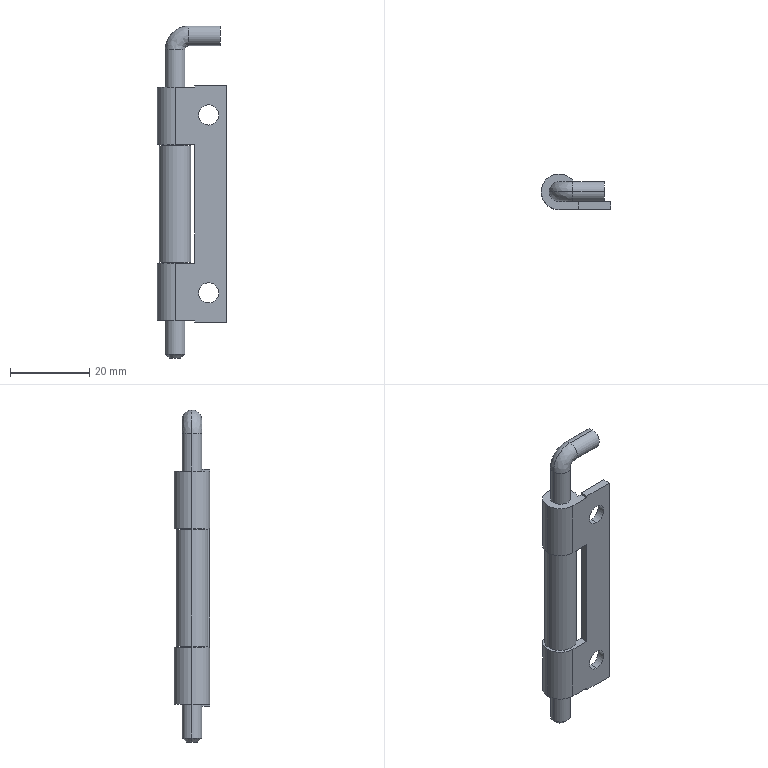Part | SolidWorks | features BaseBody 2 | 2 solids | 42 faces | box 17.6 x 9 x 84 mm | volume 4996 mm3 | cylinder 22 | plane 16 | spline 2 | cone 2 | commonest cylinder face diameters 5 x10 9 x6 5.1 x4 8 x2
STEP:
#1=CARTESIAN_POINT('',(4.5,0.,-15.));
#2=VERTEX_POINT('',#1);
#3=CARTESIAN_POINT('',(-4.5,0.,-15.));
#4=VERTEX_POINT('',#3);
#5=CARTESIAN_POINT('',(0.,0.,-15.));
#6=DIRECTION('',(0.,0.,1.));
#7=DIRECTION('',(1.,0.,0.));
#8=AXIS2_PLACEMENT_3D('',#5,#6,#7);
#9=CIRCLE('',#8,4.5);
#10=EDGE_CURVE('',#2,#4,#9,.T.);
#11=ORIENTED_EDGE('',*,*,#10,.T.);
#12=CARTESIAN_POINT('',(-4.5,0.,-0.5));
#13=VERTEX_POINT('',#12);
#14=CARTESIAN_POINT('',(-4.5,0.,0.));
#15=DIRECTION('',(0.,0.,1.));
#16=VECTOR('',#15,1000.);
#17=LINE('',#14,#16);
#18=EDGE_CURVE('',#4,#13,#17,.T.);
#19=ORIENTED_EDGE('',*,*,#18,.T.);
#20=CARTESIAN_POINT('',(4.5,0.,-0.5));
#21=VERTEX_POINT('',#20);
#22=CARTESIAN_POINT('',(0.,0.,-0.5));
#23=DIRECTION('',(0.,0.,1.));
#24=DIRECTION('',(1.,0.,0.));
#25=AXIS2_PLACEMENT_3D('',#22,#23,#24);
#26=CIRCLE('',#25,4.5);
#27=EDGE_CURVE('',#21,#13,#26,.T.);
#28=ORIENTED_EDGE('',*,*,#27,.F.);
#29=CARTESIAN_POINT('',(4.5,0.,0.));
#30=DIRECTION('',(0.,0.,1.));
#31=VECTOR('',#30,1000.);
#32=LINE('',#29,#31);
#33=EDGE_CURVE('',#2,#21,#32,.T.);
#34=ORIENTED_EDGE('',*,*,#33,.F.);
#35=EDGE_LOOP('',(#11,#19,#28,#34));
#36=FACE_OUTER_BOUND('',#35,.T.);
#37=CARTESIAN_POINT('',(0.,0.,0.));
#38=DIRECTION('',(0.,0.,1.));
#39=DIRECTION('',(1.,0.,0.));
#40=AXIS2_PLACEMENT_3D('',#37,#38,#39);
#41=CYLINDRICAL_SURFACE('',#40,4.5);
#42=ADVANCED_FACE('',(#36),#41,.T.);
#43=CARTESIAN_POINT('',(3.742,-2.5,-15.));
#44=VERTEX_POINT('',#43);
#45=CARTESIAN_POINT('',(0.,0.,-15.));
#46=DIRECTION('',(0.,0.,1.));
#47=DIRECTION('',(1.,0.,0.));
#48=AXIS2_PLACEMENT_3D('',#45,#46,#47);
#49=CIRCLE('',#48,4.5);
#50=EDGE_CURVE('',#44,#2,#49,.T.);
#51=ORIENTED_EDGE('',*,*,#50,.T.);
#52=ORIENTED_EDGE('',*,*,#33,.T.);
#53=CARTESIAN_POINT('',(3.742,-2.5,-0.5));
#54=VERTEX_POINT('',#53);
#55=CARTESIAN_POINT('',(0.,0.,-0.5));
#56=DIRECTION('',(0.,0.,1.));
#57=DIRECTION('',(1.,0.,0.));
#58=AXIS2_PLACEMENT_3D('',#55,#56,#57);
#59=CIRCLE('',#58,4.5);
#60=EDGE_CURVE('',#54,#21,#59,.T.);
#61=ORIENTED_EDGE('',*,*,#60,.F.);
#62=CARTESIAN_POINT('',(3.742,-2.5,0.));
#63=DIRECTION('',(0.,0.,-1.));
#64=VECTOR('',#63,1000.);
#65=LINE('',#62,#64);
#66=EDGE_CURVE('',#54,#44,#65,.T.);
#67=ORIENTED_EDGE('',*,*,#66,.T.);
#68=EDGE_LOOP('',(#51,#52,#61,#67));
#69=FACE_OUTER_BOUND('',#68,.T.);
#70=CARTESIAN_POINT('',(0.,0.,0.));
#71=DIRECTION('',(0.,0.,1.));
#72=DIRECTION('',(1.,0.,0.));
#73=AXIS2_PLACEMENT_3D('',#70,#71,#72);
#74=CYLINDRICAL_SURFACE('',#73,4.5);
#75=ADVANCED_FACE('',(#69),#74,.T.);
#76=CARTESIAN_POINT('',(4.5,0.,-59.5));
#77=VERTEX_POINT('',#76);
#78=CARTESIAN_POINT('',(-4.5,0.,-59.5));
#79=VERTEX_POINT('',#78);
#80=CARTESIAN_POINT('',(0.,0.,-59.5));
#81=DIRECTION('',(0.,0.,1.));
#82=DIRECTION('',(1.,0.,0.));
#83=AXIS2_PLACEMENT_3D('',#80,#81,#82);
#84=CIRCLE('',#83,4.5);
#85=EDGE_CURVE('',#77,#79,#84,.T.);
#86=ORIENTED_EDGE('',*,*,#85,.T.);
#87=CARTESIAN_POINT('',(-4.5,0.,-45.));
#88=VERTEX_POINT('',#87);
#89=CARTESIAN_POINT('',(-4.5,0.,0.));
#90=DIRECTION('',(0.,0.,1.));
#91=VECTOR('',#90,1000.);
#92=LINE('',#89,#91);
#93=EDGE_CURVE('',#79,#88,#92,.T.);
#94=ORIENTED_EDGE('',*,*,#93,.T.);
#95=CARTESIAN_POINT('',(4.5,0.,-45.));
#96=VERTEX_POINT('',#95);
#97=CARTESIAN_POINT('',(0.,0.,-45.));
#98=DIRECTION('',(0.,0.,1.));
#99=DIRECTION('',(1.,0.,0.));
#100=AXIS2_PLACEMENT_3D('',#97,#98,#99);
#101=CIRCLE('',#100,4.5);
#102=EDGE_CURVE('',#96,#88,#101,.T.);
#103=ORIENTED_EDGE('',*,*,#102,.F.);
#104=CARTESIAN_POINT('',(4.5,0.,0.));
#105=DIRECTION('',(0.,0.,1.));
#106=VECTOR('',#105,1000.);
#107=LINE('',#104,#106);
#108=EDGE_CURVE('',#77,#96,#107,.T.);
#109=ORIENTED_EDGE('',*,*,#108,.F.);
#110=EDGE_LOOP('',(#86,#94,#103,#109));
#111=FACE_OUTER_BOUND('',#110,.T.);
#112=CARTESIAN_POINT('',(0.,0.,0.));
#113=DIRECTION('',(0.,0.,1.));
#114=DIRECTION('',(1.,0.,0.));
#115=AXIS2_PLACEMENT_3D('',#112,#113,#114);
#116=CYLINDRICAL_SURFACE('',#115,4.5);
#117=ADVANCED_FACE('',(#111),#116,.T.);
#118=CARTESIAN_POINT('',(3.742,-2.5,-59.5));
#119=VERTEX_POINT('',#118);
#120=CARTESIAN_POINT('',(0.,0.,-59.5));
#121=DIRECTION('',(0.,0.,1.));
#122=DIRECTION('',(1.,0.,0.));
#123=AXIS2_PLACEMENT_3D('',#120,#121,#122);
#124=CIRCLE('',#123,4.5);
#125=EDGE_CURVE('',#119,#77,#124,.T.);
#126=ORIENTED_EDGE('',*,*,#125,.T.);
#127=ORIENTED_EDGE('',*,*,#108,.T.);
#128=CARTESIAN_POINT('',(3.742,-2.5,-45.));
#129=VERTEX_POINT('',#128);
#130=CARTESIAN_POINT('',(0.,0.,-45.));
#131=DIRECTION('',(0.,0.,1.));
#132=DIRECTION('',(1.,0.,0.));
#133=AXIS2_PLACEMENT_3D('',#130,#131,#132);
#134=CIRCLE('',#133,4.5);
#135=EDGE_CURVE('',#129,#96,#134,.T.);
#136=ORIENTED_EDGE('',*,*,#135,.F.);
#137=CARTESIAN_POINT('',(3.742,-2.5,0.));
#138=DIRECTION('',(0.,0.,-1.));
#139=VECTOR('',#138,1000.);
#140=LINE('',#137,#139);
#141=EDGE_CURVE('',#129,#119,#140,.T.);
#142=ORIENTED_EDGE('',*,*,#141,.T.);
#143=EDGE_LOOP('',(#126,#127,#136,#142));
#144=FACE_OUTER_BOUND('',#143,.T.);
#145=CARTESIAN_POINT('',(0.,0.,0.));
#146=DIRECTION('',(0.,0.,1.));
#147=DIRECTION('',(1.,0.,0.));
#148=AXIS2_PLACEMENT_3D('',#145,#146,#147);
#149=CYLINDRICAL_SURFACE('',#148,4.5);
#150=ADVANCED_FACE('',(#144),#149,.T.);
#151=CARTESIAN_POINT('',(8.5,-4.5,-4.95));
#152=VERTEX_POINT('',#151);
#153=CARTESIAN_POINT('',(8.5,-4.5,-10.05));
#154=VERTEX_POINT('',#153);
#155=CARTESIAN_POINT('',(8.5,-4.5,-7.5));
#156=DIRECTION('',(0.,-1.,0.));
#157=DIRECTION('',(0.,0.,1.));
#158=AXIS2_PLACEMENT_3D('',#155,#156,#157);
#159=CIRCLE('',#158,2.55);
#160=EDGE_CURVE('',#152,#154,#159,.T.);
#161=ORIENTED_EDGE('',*,*,#160,.T.);
#162=CARTESIAN_POINT('',(8.5,-2.5,-10.05));
#163=VERTEX_POINT('',#162);
#164=CARTESIAN_POINT('',(8.5,60.,-10.05));
#165=DIRECTION('',(0.,1.,0.));
#166=VECTOR('',#165,1000.);
#167=LINE('',#164,#166);
#168=EDGE_CURVE('',#154,#163,#167,.T.);
#169=ORIENTED_EDGE('',*,*,#168,.T.);
#170=CARTESIAN_POINT('',(8.5,-2.5,-4.95));
#171=VERTEX_POINT('',#170);
#172=CARTESIAN_POINT('',(8.5,-2.5,-7.5));
#173=DIRECTION('',(0.,-1.,0.));
#174=DIRECTION('',(0.,0.,1.));
#175=AXIS2_PLACEMENT_3D('',#172,#173,#174);
#176=CIRCLE('',#175,2.55);
#177=EDGE_CURVE('',#171,#163,#176,.T.);
#178=ORIENTED_EDGE('',*,*,#177,.F.);
#179=CARTESIAN_POINT('',(8.5,60.,-4.95));
#180=DIRECTION('',(0.,1.,0.));
#181=VECTOR('',#180,1000.);
#182=LINE('',#179,#181);
#183=EDGE_CURVE('',#152,#171,#182,.T.);
#184=ORIENTED_EDGE('',*,*,#183,.F.);
#185=EDGE_LOOP('',(#161,#169,#178,#184));
#186=FACE_OUTER_BOUND('',#185,.T.);
#187=CARTESIAN_POINT('',(8.5,60.,-7.5));
#188=DIRECTION('',(0.,1.,0.));
#189=DIRECTION('',(0.,0.,1.));
#190=AXIS2_PLACEMENT_3D('',#187,#188,#189);
#191=CYLINDRICAL_SURFACE('',#190,2.55);
#192=ADVANCED_FACE('',(#186),#191,.F.);
#193=CARTESIAN_POINT('',(8.5,-4.5,-49.95));
#194=VERTEX_POINT('',#193);
#195=CARTESIAN_POINT('',(8.5,-4.5,-55.05));
#196=VERTEX_POINT('',#195);
#197=CARTESIAN_POINT('',(8.5,-4.5,-52.5));
#198=DIRECTION('',(0.,-1.,0.));
#199=DIRECTION('',(0.,0.,1.));
#200=AXIS2_PLACEMENT_3D('',#197,#198,#199);
#201=CIRCLE('',#200,2.55);
#202=EDGE_CURVE('',#194,#196,#201,.T.);
#203=ORIENTED_EDGE('',*,*,#202,.T.);
#204=CARTESIAN_POINT('',(8.5,-2.5,-55.05));
#205=VERTEX_POINT('',#204);
#206=CARTESIAN_POINT('',(8.5,60.,-55.05));
#207=DIRECTION('',(0.,1.,0.));
#208=VECTOR('',#207,1000.);
#209=LINE('',#206,#208);
#210=EDGE_CURVE('',#196,#205,#209,.T.);
#211=ORIENTED_EDGE('',*,*,#210,.T.);
#212=CARTESIAN_POINT('',(8.5,-2.5,-49.95));
#213=VERTEX_POINT('',#212);
#214=CARTESIAN_POINT('',(8.5,-2.5,-52.5));
#215=DIRECTION('',(0.,-1.,0.));
#216=DIRECTION('',(0.,0.,1.));
#217=AXIS2_PLACEMENT_3D('',#214,#215,#216);
#218=CIRCLE('',#217,2.55);
#219=EDGE_CURVE('',#213,#205,#218,.T.);
#220=ORIENTED_EDGE('',*,*,#219,.F.);
#221=CARTESIAN_POINT('',(8.5,60.,-49.95));
#222=DIRECTION('',(0.,1.,0.));
#223=VECTOR('',#222,1000.);
#224=LINE('',#221,#223);
#225=EDGE_CURVE('',#194,#213,#224,.T.);
#226=ORIENTED_EDGE('',*,*,#225,.F.);
#227=EDGE_LOOP('',(#203,#211,#220,#226));
#228=FACE_OUTER_BOUND('',#227,.T.);
#229=CARTESIAN_POINT('',(8.5,60.,-52.5));
#230=DIRECTION('',(0.,1.,0.));
#231=DIRECTION('',(0.,0.,1.));
#232=AXIS2_PLACEMENT_3D('',#229,#230,#231);
#233=CYLINDRICAL_SURFACE('',#232,2.55);
#234=ADVANCED_FACE('',(#228),#233,.F.);
#235=CARTESIAN_POINT('',(-2.5,0.,-15.));
#236=VERTEX_POINT('',#235);
#237=CARTESIAN_POINT('',(2.5,0.,-15.));
#238=VERTEX_POINT('',#237);
#239=CARTESIAN_POINT('',(0.,0.,-15.));
#240=DIRECTION('',(0.,0.,1.));
#241=DIRECTION('',(1.,0.,0.));
#242=AXIS2_PLACEMENT_3D('',#239,#240,#241);
#243=CIRCLE('',#242,2.5);
#244=EDGE_CURVE('',#236,#238,#243,.T.);
#245=ORIENTED_EDGE('',*,*,#244,.F.);
#246=CARTESIAN_POINT('',(-2.5,0.,-0.5));
#247=VERTEX_POINT('',#246);
#248=CARTESIAN_POINT('',(-2.5,0.,0.));
#249=DIRECTION('',(0.,0.,1.));
#250=VECTOR('',#249,1000.);
#251=LINE('',#248,#250);
#252=EDGE_CURVE('',#236,#247,#251,.T.);
#253=ORIENTED_EDGE('',*,*,#252,.T.);
#254=CARTESIAN_POINT('',(2.5,0.,-0.5));
#255=VERTEX_POINT('',#254);
#256=CARTESIAN_POINT('',(0.,0.,-0.5));
#257=DIRECTION('',(0.,0.,-1.));
#258=DIRECTION('',(1.,0.,0.));
#259=AXIS2_PLACEMENT_3D('',#256,#257,#258);
#260=CIRCLE('',#259,2.5);
#261=EDGE_CURVE('',#255,#247,#260,.T.);
#262=ORIENTED_EDGE('',*,*,#261,.F.);
#263=CARTESIAN_POINT('',(2.5,0.,0.));
#264=DIRECTION('',(0.,0.,1.));
#265=VECTOR('',#264,1000.);
#266=LINE('',#263,#265);
#267=EDGE_CURVE('',#238,#255,#266,.T.);
#268=ORIENTED_EDGE('',*,*,#267,.F.);
#269=EDGE_LOOP('',(#245,#253,#262,#268));
#270=FACE_OUTER_BOUND('',#269,.T.);
#271=CARTESIAN_POINT('',(0.,0.,0.));
#272=DIRECTION('',(0.,0.,1.));
#273=DIRECTION('',(1.,0.,0.));
#274=AXIS2_PLACEMENT_3D('',#271,#272,#273);
#275=CYLINDRICAL_SURFACE('',#274,2.5);
#276=ADVANCED_FACE('',(#270),#275,.F.);
#277=CARTESIAN_POINT('',(-2.5,0.,-59.5));
#278=VERTEX_POINT('',#277);
#279=CARTESIAN_POINT('',(2.5,0.,-59.5));
#280=VERTEX_POINT('',#279);
#281=CARTESIAN_POINT('',(0.,0.,-59.5));
#282=DIRECTION('',(0.,0.,1.));
#283=DIRECTION('',(1.,0.,0.));
#284=AXIS2_PLACEMENT_3D('',#281,#282,#283);
#285=CIRCLE('',#284,2.5);
#286=EDGE_CURVE('',#278,#280,#285,.T.);
#287=ORIENTED_EDGE('',*,*,#286,.F.);
#288=CARTESIAN_POINT('',(-2.5,0.,-45.));
#289=VERTEX_POINT('',#288);
#290=CARTESIAN_POINT('',(-2.5,0.,0.));
#291=DIRECTION('',(0.,0.,1.));
#292=VECTOR('',#291,1000.);
#293=LINE('',#290,#292);
#294=EDGE_CURVE('',#278,#289,#293,.T.);
#295=ORIENTED_EDGE('',*,*,#294,.T.);
#296=CARTESIAN_POINT('',(2.5,0.,-45.));
#297=VERTEX_POINT('',#296);
#298=CARTESIAN_POINT('',(0.,0.,-45.));
#299=DIRECTION('',(0.,0.,-1.));
#300=DIRECTION('',(1.,0.,0.));
#301=AXIS2_PLACEMENT_3D('',#298,#299,#300);
#302=CIRCLE('',#301,2.5);
#303=EDGE_CURVE('',#297,#289,#302,.T.);
#304=ORIENTED_EDGE('',*,*,#303,.F.);
#305=CARTESIAN_POINT('',(2.5,0.,0.));
#306=DIRECTION('',(0.,0.,1.));
#307=VECTOR('',#306,1000.);
#308=LINE('',#305,#307);
#309=EDGE_CURVE('',#280,#297,#308,.T.);
#310=ORIENTED_EDGE('',*,*,#309,.F.);
#311=EDGE_LOOP('',(#287,#295,#304,#310));
#312=FACE_OUTER_BOUND('',#311,.T.);
#313=CARTESIAN_POINT('',(0.,0.,0.));
#314=DIRECTION('',(0.,0.,1.));
#315=DIRECTION('',(1.,0.,0.));
#316=AXIS2_PLACEMENT_3D('',#313,#314,#315);
#317=CYLINDRICAL_SURFACE('',#316,2.5);
#318=ADVANCED_FACE('',(#312),#317,.F.);
#319=CARTESIAN_POINT('',(0.,-4.5,-0.5));
#320=VERTEX_POINT('',#319);
#321=CARTESIAN_POINT('',(5.,-4.5,-0.5));
#322=VERTEX_POINT('',#321);
#323=CARTESIAN_POINT('',(0.,-4.5,-0.5));
#324=DIRECTION('',(1.,0.,0.));
#325=VECTOR('',#324,1000.);
#326=LINE('',#323,#325);
#327=EDGE_CURVE('',#320,#322,#326,.T.);
#328=ORIENTED_EDGE('',*,*,#327,.F.);
#329=CARTESIAN_POINT('',(0.,-4.5,-15.));
#330=VERTEX_POINT('',#329);
#331=CARTESIAN_POINT('',(0.,-4.5,0.));
#332=DIRECTION('',(0.,0.,1.));
#333=VECTOR('',#332,1000.);
#334=LINE('',#331,#333);
#335=EDGE_CURVE('',#330,#320,#334,.T.);
#336=ORIENTED_EDGE('',*,*,#335,.F.);
#337=CARTESIAN_POINT('',(5.,-4.5,-15.));
#338=VERTEX_POINT('',#337);
#339=CARTESIAN_POINT('',(0.,-4.5,-15.));
#340=DIRECTION('',(-1.,0.,0.));
#341=VECTOR('',#340,1000.);
#342=LINE('',#339,#341);
#343=EDGE_CURVE('',#338,#330,#342,.T.);
#344=ORIENTED_EDGE('',*,*,#343,.F.);
#345=CARTESIAN_POINT('',(5.,-4.5,-45.));
#346=VERTEX_POINT('',#345);
#347=CARTESIAN_POINT('',(5.,-4.5,0.));
#348=DIRECTION('',(0.,0.,1.));
#349=VECTOR('',#348,1000.);
#350=LINE('',#347,#349);
#351=EDGE_CURVE('',#346,#338,#350,.T.);
#352=ORIENTED_EDGE('',*,*,#351,.F.);
#353=CARTESIAN_POINT('',(0.,-4.5,-45.));
#354=VERTEX_POINT('',#353);
#355=CARTESIAN_POINT('',(0.,-4.5,-45.));
#356=DIRECTION('',(1.,0.,0.));
#357=VECTOR('',#356,1000.);
#358=LINE('',#355,#357);
#359=EDGE_CURVE('',#354,#346,#358,.T.);
#360=ORIENTED_EDGE('',*,*,#359,.F.);
#361=CARTESIAN_POINT('',(0.,-4.5,-59.5));
#362=VERTEX_POINT('',#361);
#363=CARTESIAN_POINT('',(0.,-4.5,0.));
#364=DIRECTION('',(0.,0.,1.));
#365=VECTOR('',#364,1000.);
#366=LINE('',#363,#365);
#367=EDGE_CURVE('',#362,#354,#366,.T.);
#368=ORIENTED_EDGE('',*,*,#367,.F.);
#369=CARTESIAN_POINT('',(5.,-4.5,-59.5));
#370=VERTEX_POINT('',#369);
#371=CARTESIAN_POINT('',(0.,-4.5,-59.5));
#372=DIRECTION('',(-1.,0.,0.));
#373=VECTOR('',#372,1000.);
#374=LINE('',#371,#373);
#375=EDGE_CURVE('',#370,#362,#374,.T.);
#376=ORIENTED_EDGE('',*,*,#375,.F.);
#377=CARTESIAN_POINT('',(5.,-4.5,-60.));
#378=VERTEX_POINT('',#377);
#379=CARTESIAN_POINT('',(5.,-4.5,-59.5));
#380=DIRECTION('',(0.,0.,1.));
#381=VECTOR('',#380,1000.);
#382=LINE('',#379,#381);
#383=EDGE_CURVE('',#378,#370,#382,.T.);
#384=ORIENTED_EDGE('',*,*,#383,.F.);
#385=CARTESIAN_POINT('',(13.1,-4.5,-60.));
#386=VERTEX_POINT('',#385);
#387=CARTESIAN_POINT('',(0.,-4.5,-60.));
#388=DIRECTION('',(-1.,0.,0.));
#389=VECTOR('',#388,1000.);
#390=LINE('',#387,#389);
#391=EDGE_CURVE('',#386,#378,#390,.T.);
#392=ORIENTED_EDGE('',*,*,#391,.F.);
#393=CARTESIAN_POINT('',(13.1,-4.5,0.));
#394=VERTEX_POINT('',#393);
#395=CARTESIAN_POINT('',(13.1,-4.5,0.));
#396=DIRECTION('',(0.,0.,-1.));
#397=VECTOR('',#396,1000.);
#398=LINE('',#395,#397);
#399=EDGE_CURVE('',#394,#386,#398,.T.);
#400=ORIENTED_EDGE('',*,*,#399,.F.);
#401=CARTESIAN_POINT('',(5.,-4.5,0.));
#402=VERTEX_POINT('',#401);
#403=CARTESIAN_POINT('',(0.,-4.5,0.));
#404=DIRECTION('',(1.,0.,0.));
#405=VECTOR('',#404,1000.);
#406=LINE('',#403,#405);
#407=EDGE_CURVE('',#402,#394,#406,.T.);
#408=ORIENTED_EDGE('',*,*,#407,.F.);
#409=CARTESIAN_POINT('',(5.,-4.5,0.));
#410=DIRECTION('',(0.,0.,1.));
#411=VECTOR('',#410,1000.);
#412=LINE('',#409,#411);
#413=EDGE_CURVE('',#322,#402,#412,.T.);
#414=ORIENTED_EDGE('',*,*,#413,.F.);
#415=EDGE_LOOP('',(#328,#336,#344,#352,#360,#368,#376,#384,#392,#400,#408,#414));
#416=FACE_OUTER_BOUND('',#415,.T.);
#417=ORIENTED_EDGE('',*,*,#160,.F.);
#418=CARTESIAN_POINT('',(8.5,-4.5,-7.5));
#419=DIRECTION('',(0.,-1.,0.));
#420=DIRECTION('',(0.,0.,1.));
#421=AXIS2_PLACEMENT_3D('',#418,#419,#420);
#422=CIRCLE('',#421,2.55);
#423=EDGE_CURVE('',#154,#152,#422,.T.);
#424=ORIENTED_EDGE('',*,*,#423,.F.);
#425=EDGE_LOOP('',(#417,#424));
#426=FACE_BOUND('',#425,.T.);
#427=ORIENTED_EDGE('',*,*,#202,.F.);
#428=CARTESIAN_POINT('',(8.5,-4.5,-52.5));
#429=DIRECTION('',(0.,-1.,0.));
#430=DIRECTION('',(0.,0.,1.));
#431=AXIS2_PLACEMENT_3D('',#428,#429,#430);
#432=CIRCLE('',#431,2.55);
#433=EDGE_CURVE('',#196,#194,#432,.T.);
#434=ORIENTED_EDGE('',*,*,#433,.F.);
#435=EDGE_LOOP('',(#427,#434));
#436=FACE_BOUND('',#435,.T.);
#437=CARTESIAN_POINT('',(0.,-4.5,0.));
#438=DIRECTION('',(0.,1.,0.));
#439=DIRECTION('',(0.,0.,1.));
#440=AXIS2_PLACEMENT_3D('',#437,#438,#439);
#441=PLANE('',#440);
#442=ADVANCED_FACE('',(#416,#426,#436),#441,.F.);
#443=ORIENTED_EDGE('',*,*,#327,.T.);
#444=CARTESIAN_POINT('',(5.,-2.5,-0.5));
#445=VERTEX_POINT('',#444);
#446=CARTESIAN_POINT('',(5.,60.,-0.5));
#447=DIRECTION('',(0.,1.,0.));
#448=VECTOR('',#447,1000.);
#449=LINE('',#446,#448);
#450=EDGE_CURVE('',#322,#445,#449,.T.);
#451=ORIENTED_EDGE('',*,*,#450,.T.);
#452=CARTESIAN_POINT('',(13.1,-2.5,-0.5));
#453=DIRECTION('',(-1.,0.,0.));
#454=VECTOR('',#453,1000.);
#455=LINE('',#452,#454);
#456=EDGE_CURVE('',#445,#54,#455,.T.);
#457=ORIENTED_EDGE('',*,*,#456,.T.);
#458=ORIENTED_EDGE('',*,*,#60,.T.);
#459=ORIENTED_EDGE('',*,*,#27,.T.);
#460=CARTESIAN_POINT('',(0.,0.,-0.5));
#461=DIRECTION('',(0.,0.,1.));
#462=DIRECTION('',(1.,0.,0.));
#463=AXIS2_PLACEMENT_3D('',#460,#461,#462);
#464=CIRCLE('',#463,4.5);
#465=EDGE_CURVE('',#13,#320,#464,.T.);
#466=ORIENTED_EDGE('',*,*,#465,.T.);
#467=EDGE_LOOP('',(#443,#451,#457,#458,#459,#466));
#468=FACE_OUTER_BOUND('',#467,.T.);
#469=ORIENTED_EDGE('',*,*,#261,.T.);
#470=CARTESIAN_POINT('',(0.,0.,-0.5));
#471=DIRECTION('',(0.,0.,-1.));
#472=DIRECTION('',(1.,0.,0.));
#473=AXIS2_PLACEMENT_3D('',#470,#471,#472);
#474=CIRCLE('',#473,2.5);
#475=EDGE_CURVE('',#247,#255,#474,.T.);
#476=ORIENTED_EDGE('',*,*,#475,.T.);
#477=EDGE_LOOP('',(#469,#476));
#478=FACE_BOUND('',#477,.T.);
#479=CARTESIAN_POINT('',(5.,60.,-0.5));
#480=DIRECTION('',(0.,0.,1.));
#481=DIRECTION('',(1.,0.,0.));
#482=AXIS2_PLACEMENT_3D('',#479,#480,#481);
#483=PLANE('',#482);
#484=ADVANCED_FACE('',(#468,#478),#483,.T.);
#485=ORIENTED_EDGE('',*,*,#18,.F.);
#486=CARTESIAN_POINT('',(0.,0.,-15.));
#487=DIRECTION('',(0.,0.,1.));
#488=DIRECTION('',(1.,0.,0.));
#489=AXIS2_PLACEMENT_3D('',#486,#487,#488);
#490=CIRCLE('',#489,4.5);
#491=EDGE_CURVE('',#4,#330,#490,.T.);
#492=ORIENTED_EDGE('',*,*,#491,.T.);
#493=ORIENTED_EDGE('',*,*,#335,.T.);
#494=ORIENTED_EDGE('',*,*,#465,.F.);
#495=EDGE_LOOP('',(#485,#492,#493,#494));
#496=FACE_OUTER_BOUND('',#495,.T.);
#497=CARTESIAN_POINT('',(0.,0.,0.));
#498=DIRECTION('',(0.,0.,1.));
#499=DIRECTION('',(1.,0.,0.));
#500=AXIS2_PLACEMENT_3D('',#497,#498,#499);
#501=CYLINDRICAL_SURFACE('',#500,4.5);
#502=ADVANCED_FACE('',(#496),#501,.T.);
#503=ORIENTED_EDGE('',*,*,#343,.T.);
#504=ORIENTED_EDGE('',*,*,#491,.F.);
#505=ORIENTED_EDGE('',*,*,#10,.F.);
#506=ORIENTED_EDGE('',*,*,#50,.F.);
#507=CARTESIAN_POINT('',(5.,-2.5,-15.));
#508=VERTEX_POINT('',#507);
#509=CARTESIAN_POINT('',(-15.,-2.5,-15.));
#510=DIRECTION('',(1.,0.,0.));
#511=VECTOR('',#510,1000.);
#512=LINE('',#509,#511);
#513=EDGE_CURVE('',#44,#508,#512,.T.);
#514=ORIENTED_EDGE('',*,*,#513,.T.);
#515=CARTESIAN_POINT('',(5.,60.,-15.));
#516=DIRECTION('',(0.,-1.,0.));
#517=VECTOR('',#516,1000.);
#518=LINE('',#515,#517);
#519=EDGE_CURVE('',#508,#338,#518,.T.);
#520=ORIENTED_EDGE('',*,*,#519,.T.);
#521=EDGE_LOOP('',(#503,#504,#505,#506,#514,#520));
#522=FACE_OUTER_BOUND('',#521,.T.);
#523=CARTESIAN_POINT('',(0.,0.,-15.));
#524=DIRECTION('',(0.,0.,1.));
#525=DIRECTION('',(1.,0.,0.));
#526=AXIS2_PLACEMENT_3D('',#523,#524,#525);
#527=CIRCLE('',#526,2.5);
#528=EDGE_CURVE('',#238,#236,#527,.T.);
#529=ORIENTED_EDGE('',*,*,#528,.T.);
#530=ORIENTED_EDGE('',*,*,#244,.T.);
#531=EDGE_LOOP('',(#529,#530));
#532=FACE_BOUND('',#531,.T.);
#533=CARTESIAN_POINT('',(-15.,60.,-15.));
#534=DIRECTION('',(0.,0.,-1.));
#535=DIRECTION('',(-1.,0.,0.));
#536=AXIS2_PLACEMENT_3D('',#533,#534,#535);
#537=PLANE('',#536);
#538=ADVANCED_FACE('',(#522,#532),#537,.T.);
#539=ORIENTED_EDGE('',*,*,#351,.T.);
#540=ORIENTED_EDGE('',*,*,#519,.F.);
#541=CARTESIAN_POINT('',(5.,-2.5,-45.));
#542=VERTEX_POINT('',#541);
#543=CARTESIAN_POINT('',(5.,-2.5,-15.));
#544=DIRECTION('',(0.,0.,-1.));
#545=VECTOR('',#544,1000.);
#546=LINE('',#543,#545);
#547=EDGE_CURVE('',#508,#542,#546,.T.);
#548=ORIENTED_EDGE('',*,*,#547,.T.);
#549=CARTESIAN_POINT('',(5.,60.,-45.));
#550=DIRECTION('',(0.,-1.,0.));
#551=VECTOR('',#550,1000.);
#552=LINE('',#549,#551);
#553=EDGE_CURVE('',#542,#346,#552,.T.);
#554=ORIENTED_EDGE('',*,*,#553,.T.);
#555=EDGE_LOOP('',(#539,#540,#548,#554));
#556=FACE_OUTER_BOUND('',#555,.T.);
#557=CARTESIAN_POINT('',(5.,60.,-15.));
#558=DIRECTION('',(-1.,0.,0.));
#559=DIRECTION('',(0.,0.,1.));
#560=AXIS2_PLACEMENT_3D('',#557,#558,#559);
#561=PLANE('',#560);
#562=ADVANCED_FACE('',(#556),#561,.T.);
#563=ORIENTED_EDGE('',*,*,#359,.T.);
#564=ORIENTED_EDGE('',*,*,#553,.F.);
#565=CARTESIAN_POINT('',(5.,-2.5,-45.));
#566=DIRECTION('',(-1.,0.,0.));
#567=VECTOR('',#566,1000.);
#568=LINE('',#565,#567);
#569=EDGE_CURVE('',#542,#129,#568,.T.);
#570=ORIENTED_EDGE('',*,*,#569,.T.);
#571=ORIENTED_EDGE('',*,*,#135,.T.);
#572=ORIENTED_EDGE('',*,*,#102,.T.);
#573=CARTESIAN_POINT('',(0.,0.,-45.));
#574=DIRECTION('',(0.,0.,1.));
#575=DIRECTION('',(1.,0.,0.));
#576=AXIS2_PLACEMENT_3D('',#573,#574,#575);
#577=CIRCLE('',#576,4.5);
#578=EDGE_CURVE('',#88,#354,#577,.T.);
#579=ORIENTED_EDGE('',*,*,#578,.T.);
#580=EDGE_LOOP('',(#563,#564,#570,#571,#572,#579));
#581=FACE_OUTER_BOUND('',#580,.T.);
#582=ORIENTED_EDGE('',*,*,#303,.T.);
#583=CARTESIAN_POINT('',(0.,0.,-45.));
#584=DIRECTION('',(0.,0.,-1.));
#585=DIRECTION('',(1.,0.,0.));
#586=AXIS2_PLACEMENT_3D('',#583,#584,#585);
#587=CIRCLE('',#586,2.5);
#588=EDGE_CURVE('',#289,#297,#587,.T.);
#589=ORIENTED_EDGE('',*,*,#588,.T.);
#590=EDGE_LOOP('',(#582,#589));
#591=FACE_BOUND('',#590,.T.);
#592=CARTESIAN_POINT('',(5.,60.,-45.));
#593=DIRECTION('',(0.,0.,1.));
#594=DIRECTION('',(1.,0.,0.));
#595=AXIS2_PLACEMENT_3D('',#592,#593,#594);
#596=PLANE('',#595);
#597=ADVANCED_FACE('',(#581,#591),#596,.T.);
#598=ORIENTED_EDGE('',*,*,#93,.F.);
#599=CARTESIAN_POINT('',(0.,0.,-59.5));
#600=DIRECTION('',(0.,0.,1.));
#601=DIRECTION('',(1.,0.,0.));
#602=AXIS2_PLACEMENT_3D('',#599,#600,#601);
#603=CIRCLE('',#602,4.5);
#604=EDGE_CURVE('',#79,#362,#603,.T.);
#605=ORIENTED_EDGE('',*,*,#604,.T.);
#606=ORIENTED_EDGE('',*,*,#367,.T.);
#607=ORIENTED_EDGE('',*,*,#578,.F.);
#608=EDGE_LOOP('',(#598,#605,#606,#607));
#609=FACE_OUTER_BOUND('',#608,.T.);
#610=CARTESIAN_POINT('',(0.,0.,0.));
#611=DIRECTION('',(0.,0.,1.));
#612=DIRECTION('',(1.,0.,0.));
#613=AXIS2_PLACEMENT_3D('',#610,#611,#612);
#614=CYLINDRICAL_SURFACE('',#613,4.5);
#615=ADVANCED_FACE('',(#609),#614,.T.);
#616=ORIENTED_EDGE('',*,*,#375,.T.);
#617=ORIENTED_EDGE('',*,*,#604,.F.);
#618=ORIENTED_EDGE('',*,*,#85,.F.);
#619=ORIENTED_EDGE('',*,*,#125,.F.);
#620=CARTESIAN_POINT('',(5.,-2.5,-59.5));
#621=VERTEX_POINT('',#620);
#622=CARTESIAN_POINT('',(-15.,-2.5,-59.5));
#623=DIRECTION('',(1.,0.,0.));
#624=VECTOR('',#623,1000.);
#625=LINE('',#622,#624);
#626=EDGE_CURVE('',#119,#621,#625,.T.);
#627=ORIENTED_EDGE('',*,*,#626,.T.);
#628=CARTESIAN_POINT('',(5.,60.,-59.5));
#629=DIRECTION('',(0.,-1.,0.));
#630=VECTOR('',#629,1000.);
#631=LINE('',#628,#630);
#632=EDGE_CURVE('',#621,#370,#631,.T.);
#633=ORIENTED_EDGE('',*,*,#632,.T.);
#634=EDGE_LOOP('',(#616,#617,#618,#619,#627,#633));
#635=FACE_OUTER_BOUND('',#634,.T.);
#636=CARTESIAN_POINT('',(0.,0.,-59.5));
#637=DIRECTION('',(0.,0.,1.));
#638=DIRECTION('',(1.,0.,0.));
#639=AXIS2_PLACEMENT_3D('',#636,#637,#638);
#640=CIRCLE('',#639,2.5);
#641=EDGE_CURVE('',#280,#278,#640,.T.);
#642=ORIENTED_EDGE('',*,*,#641,.T.);
#643=ORIENTED_EDGE('',*,*,#286,.T.);
#644=EDGE_LOOP('',(#642,#643));
#645=FACE_BOUND('',#644,.T.);
#646=CARTESIAN_POINT('',(-15.,60.,-59.5));
#647=DIRECTION('',(0.,0.,-1.));
#648=DIRECTION('',(-1.,0.,0.));
#649=AXIS2_PLACEMENT_3D('',#646,#647,#648);
#650=PLANE('',#649);
#651=ADVANCED_FACE('',(#635,#645),#650,.T.);
#652=CARTESIAN_POINT('',(13.1,-2.5,-60.));
#653=VERTEX_POINT('',#652);
#654=CARTESIAN_POINT('',(5.,-2.5,-60.));
#655=VERTEX_POINT('',#654);
#656=CARTESIAN_POINT('',(0.,-2.5,-60.));
#657=DIRECTION('',(-1.,0.,0.));
#658=VECTOR('',#657,1000.);
#659=LINE('',#656,#658);
#660=EDGE_CURVE('',#653,#655,#659,.T.);
#661=ORIENTED_EDGE('',*,*,#660,.F.);
#662=CARTESIAN_POINT('',(13.1,0.,-60.));
#663=DIRECTION('',(0.,1.,0.));
#664=VECTOR('',#663,1000.);
#665=LINE('',#662,#664);
#666=EDGE_CURVE('',#386,#653,#665,.T.);
#667=ORIENTED_EDGE('',*,*,#666,.F.);
#668=ORIENTED_EDGE('',*,*,#391,.T.);
#669=CARTESIAN_POINT('',(5.,0.,-60.));
#670=DIRECTION('',(0.,-1.,0.));
#671=VECTOR('',#670,1000.);
#672=LINE('',#669,#671);
#673=EDGE_CURVE('',#655,#378,#672,.T.);
#674=ORIENTED_EDGE('',*,*,#673,.F.);
#675=EDGE_LOOP('',(#661,#667,#668,#674));
#676=FACE_OUTER_BOUND('',#675,.T.);
#677=CARTESIAN_POINT('',(0.,0.,-60.));
#678=DIRECTION('',(0.,0.,1.));
#679=DIRECTION('',(1.,0.,0.));
#680=AXIS2_PLACEMENT_3D('',#677,#678,#679);
#681=PLANE('',#680);
#682=ADVANCED_FACE('',(#676),#681,.F.);
#683=CARTESIAN_POINT('',(13.1,-2.5,0.));
#684=VERTEX_POINT('',#683);
#685=CARTESIAN_POINT('',(13.1,-2.5,0.));
#686=DIRECTION('',(0.,0.,-1.));
#687=VECTOR('',#686,1000.);
#688=LINE('',#685,#687);
#689=EDGE_CURVE('',#684,#653,#688,.T.);
#690=ORIENTED_EDGE('',*,*,#689,.F.);
#691=CARTESIAN_POINT('',(13.1,-4.5,0.));
#692=DIRECTION('',(0.,1.,0.));
#693=VECTOR('',#692,1000.);
#694=LINE('',#691,#693);
#695=EDGE_CURVE('',#394,#684,#694,.T.);
#696=ORIENTED_EDGE('',*,*,#695,.F.);
#697=ORIENTED_EDGE('',*,*,#399,.T.);
#698=ORIENTED_EDGE('',*,*,#666,.T.);
#699=EDGE_LOOP('',(#690,#696,#697,#698));
#700=FACE_OUTER_BOUND('',#699,.T.);
#701=CARTESIAN_POINT('',(13.1,-4.5,0.));
#702=DIRECTION('',(-1.,0.,0.));
#703=DIRECTION('',(0.,0.,1.));
#704=AXIS2_PLACEMENT_3D('',#701,#702,#703);
#705=PLANE('',#704);
#706=ADVANCED_FACE('',(#700),#705,.F.);
#707=ORIENTED_EDGE('',*,*,#407,.T.);
#708=ORIENTED_EDGE('',*,*,#695,.T.);
#709=CARTESIAN_POINT('',(5.,-2.5,0.));
#710=VERTEX_POINT('',#709);
#711=CARTESIAN_POINT('',(0.,-2.5,0.));
#712=DIRECTION('',(-1.,0.,0.));
#713=VECTOR('',#712,1000.);
#714=LINE('',#711,#713);
#715=EDGE_CURVE('',#684,#710,#714,.T.);
#716=ORIENTED_EDGE('',*,*,#715,.T.);
#717=CARTESIAN_POINT('',(5.,0.,0.));
#718=DIRECTION('',(0.,-1.,0.));
#719=VECTOR('',#718,1000.);
#720=LINE('',#717,#719);
#721=EDGE_CURVE('',#710,#402,#720,.T.);
#722=ORIENTED_EDGE('',*,*,#721,.T.);
#723=EDGE_LOOP('',(#707,#708,#716,#722));
#724=FACE_OUTER_BOUND('',#723,.T.);
#725=CARTESIAN_POINT('',(0.,0.,0.));
#726=DIRECTION('',(0.,0.,1.));
#727=DIRECTION('',(1.,0.,0.));
#728=AXIS2_PLACEMENT_3D('',#725,#726,#727);
#729=PLANE('',#728);
#730=ADVANCED_FACE('',(#724),#729,.T.);
#731=ORIENTED_EDGE('',*,*,#168,.F.);
#732=ORIENTED_EDGE('',*,*,#423,.T.);
#733=ORIENTED_EDGE('',*,*,#183,.T.);
#734=CARTESIAN_POINT('',(8.5,-2.5,-7.5));
#735=DIRECTION('',(0.,-1.,0.));
#736=DIRECTION('',(0.,0.,1.));
#737=AXIS2_PLACEMENT_3D('',#734,#735,#736);
#738=CIRCLE('',#737,2.55);
#739=EDGE_CURVE('',#163,#171,#738,.T.);
#740=ORIENTED_EDGE('',*,*,#739,.F.);
#741=EDGE_LOOP('',(#731,#732,#733,#740));
#742=FACE_OUTER_BOUND('',#741,.T.);
#743=CARTESIAN_POINT('',(8.5,60.,-7.5));
#744=DIRECTION('',(0.,1.,0.));
#745=DIRECTION('',(0.,0.,1.));
#746=AXIS2_PLACEMENT_3D('',#743,#744,#745);
#747=CYLINDRICAL_SURFACE('',#746,2.55);
#748=ADVANCED_FACE('',(#742),#747,.F.);
#749=ORIENTED_EDGE('',*,*,#210,.F.);
#750=ORIENTED_EDGE('',*,*,#433,.T.);
#751=ORIENTED_EDGE('',*,*,#225,.T.);
#752=CARTESIAN_POINT('',(8.5,-2.5,-52.5));
#753=DIRECTION('',(0.,-1.,0.));
#754=DIRECTION('',(0.,0.,1.));
#755=AXIS2_PLACEMENT_3D('',#752,#753,#754);
#756=CIRCLE('',#755,2.55);
#757=EDGE_CURVE('',#205,#213,#756,.T.);
#758=ORIENTED_EDGE('',*,*,#757,.F.);
#759=EDGE_LOOP('',(#749,#750,#751,#758));
#760=FACE_OUTER_BOUND('',#759,.T.);
#761=CARTESIAN_POINT('',(8.5,60.,-52.5));
#762=DIRECTION('',(0.,1.,0.));
#763=DIRECTION('',(0.,0.,1.));
#764=AXIS2_PLACEMENT_3D('',#761,#762,#763);
#765=CYLINDRICAL_SURFACE('',#764,2.55);
#766=ADVANCED_FACE('',(#760),#765,.F.);
#767=ORIENTED_EDGE('',*,*,#413,.T.);
#768=ORIENTED_EDGE('',*,*,#721,.F.);
#769=CARTESIAN_POINT('',(5.,-2.5,0.));
#770=DIRECTION('',(0.,0.,-1.));
#771=VECTOR('',#770,1000.);
#772=LINE('',#769,#771);
#773=EDGE_CURVE('',#710,#445,#772,.T.);
#774=ORIENTED_EDGE('',*,*,#773,.T.);
#775=ORIENTED_EDGE('',*,*,#450,.F.);
#776=EDGE_LOOP('',(#767,#768,#774,#775));
#777=FACE_OUTER_BOUND('',#776,.T.);
#778=CARTESIAN_POINT('',(5.,60.,0.));
#779=DIRECTION('',(-1.,0.,0.));
#780=DIRECTION('',(0.,0.,1.));
#781=AXIS2_PLACEMENT_3D('',#778,#779,#780);
#782=PLANE('',#781);
#783=ADVANCED_FACE('',(#777),#782,.T.);
#784=ORIENTED_EDGE('',*,*,#252,.F.);
#785=ORIENTED_EDGE('',*,*,#528,.F.);
#786=ORIENTED_EDGE('',*,*,#267,.T.);
#787=ORIENTED_EDGE('',*,*,#475,.F.);
#788=EDGE_LOOP('',(#784,#785,#786,#787));
#789=FACE_OUTER_BOUND('',#788,.T.);
#790=CARTESIAN_POINT('',(0.,0.,0.));
#791=DIRECTION('',(0.,0.,1.));
#792=DIRECTION('',(1.,0.,0.));
#793=AXIS2_PLACEMENT_3D('',#790,#791,#792);
#794=CYLINDRICAL_SURFACE('',#793,2.5);
#795=ADVANCED_FACE('',(#789),#794,.F.);
#796=ORIENTED_EDGE('',*,*,#715,.F.);
#797=ORIENTED_EDGE('',*,*,#689,.T.);
#798=ORIENTED_EDGE('',*,*,#660,.T.);
#799=CARTESIAN_POINT('',(5.,-2.5,0.));
#800=DIRECTION('',(0.,0.,-1.));
#801=VECTOR('',#800,1000.);
#802=LINE('',#799,#801);
#803=EDGE_CURVE('',#621,#655,#802,.T.);
#804=ORIENTED_EDGE('',*,*,#803,.F.);
#805=ORIENTED_EDGE('',*,*,#626,.F.);
#806=ORIENTED_EDGE('',*,*,#141,.F.);
#807=ORIENTED_EDGE('',*,*,#569,.F.);
#808=ORIENTED_EDGE('',*,*,#547,.F.);
#809=ORIENTED_EDGE('',*,*,#513,.F.);
#810=ORIENTED_EDGE('',*,*,#66,.F.);
#811=ORIENTED_EDGE('',*,*,#456,.F.);
#812=ORIENTED_EDGE('',*,*,#773,.F.);
#813=EDGE_LOOP('',(#796,#797,#798,#804,#805,#806,#807,#808,#809,#810,#811,#812));
#814=FACE_OUTER_BOUND('',#813,.T.);
#815=ORIENTED_EDGE('',*,*,#177,.T.);
#816=ORIENTED_EDGE('',*,*,#739,.T.);
#817=EDGE_LOOP('',(#815,#816));
#818=FACE_BOUND('',#817,.T.);
#819=ORIENTED_EDGE('',*,*,#219,.T.);
#820=ORIENTED_EDGE('',*,*,#757,.T.);
#821=EDGE_LOOP('',(#819,#820));
#822=FACE_BOUND('',#821,.T.);
#823=CARTESIAN_POINT('',(13.1,-2.5,0.));
#824=DIRECTION('',(0.,-1.,0.));
#825=DIRECTION('',(0.,0.,-1.));
#826=AXIS2_PLACEMENT_3D('',#823,#824,#825);
#827=PLANE('',#826);
#828=ADVANCED_FACE('',(#814,#818,#822),#827,.F.);
#829=ORIENTED_EDGE('',*,*,#294,.F.);
#830=ORIENTED_EDGE('',*,*,#641,.F.);
#831=ORIENTED_EDGE('',*,*,#309,.T.);
#832=ORIENTED_EDGE('',*,*,#588,.F.);
#833=EDGE_LOOP('',(#829,#830,#831,#832));
#834=FACE_OUTER_BOUND('',#833,.T.);
#835=CARTESIAN_POINT('',(0.,0.,0.));
#836=DIRECTION('',(0.,0.,1.));
#837=DIRECTION('',(1.,0.,0.));
#838=AXIS2_PLACEMENT_3D('',#835,#836,#837);
#839=CYLINDRICAL_SURFACE('',#838,2.5);
#840=ADVANCED_FACE('',(#834),#839,.F.);
#841=ORIENTED_EDGE('',*,*,#383,.T.);
#842=ORIENTED_EDGE('',*,*,#632,.F.);
#843=ORIENTED_EDGE('',*,*,#803,.T.);
#844=ORIENTED_EDGE('',*,*,#673,.T.);
#845=EDGE_LOOP('',(#841,#842,#843,#844));
#846=FACE_OUTER_BOUND('',#845,.T.);
#847=CARTESIAN_POINT('',(5.,60.,-59.5));
#848=DIRECTION('',(-1.,0.,0.));
#849=DIRECTION('',(0.,0.,1.));
#850=AXIS2_PLACEMENT_3D('',#847,#848,#849);
#851=PLANE('',#850);
#852=ADVANCED_FACE('',(#846),#851,.T.);
#853=CLOSED_SHELL('',(#42,#75,#117,#150,#192,#234,#276,#318,#442,#484,#502,#538,#562,#597,#615,#651,#682,#706,#730,#748,#766,#783,#795,#828,#840,#852));
#854=MANIFOLD_SOLID_BREP('',#853);
#855=CARTESIAN_POINT('',(4.,0.,-15.25));
#856=VERTEX_POINT('',#855);
#857=CARTESIAN_POINT('',(-4.,0.,-15.25));
#858=VERTEX_POINT('',#857);
#859=CARTESIAN_POINT('',(0.,0.,-15.25));
#860=DIRECTION('',(0.,0.,-1.));
#861=DIRECTION('',(1.,0.,0.));
#862=AXIS2_PLACEMENT_3D('',#859,#860,#861);
#863=CIRCLE('',#862,4.);
#864=EDGE_CURVE('',#856,#858,#863,.T.);
#865=ORIENTED_EDGE('',*,*,#864,.T.);
#866=CARTESIAN_POINT('',(-4.,0.,-44.75));
#867=VERTEX_POINT('',#866);
#868=CARTESIAN_POINT('',(-4.,0.,-44.75));
#869=DIRECTION('',(0.,0.,-1.));
#870=VECTOR('',#869,1000.);
#871=LINE('',#868,#870);
#872=EDGE_CURVE('',#858,#867,#871,.T.);
#873=ORIENTED_EDGE('',*,*,#872,.T.);
#874=CARTESIAN_POINT('',(4.,0.,-44.75));
#875=VERTEX_POINT('',#874);
#876=CARTESIAN_POINT('',(0.,0.,-44.75));
#877=DIRECTION('',(0.,0.,1.));
#878=DIRECTION('',(1.,0.,0.));
#879=AXIS2_PLACEMENT_3D('',#876,#877,#878);
#880=CIRCLE('',#879,4.);
#881=EDGE_CURVE('',#867,#875,#880,.T.);
#882=ORIENTED_EDGE('',*,*,#881,.T.);
#883=CARTESIAN_POINT('',(4.,0.,-44.75));
#884=DIRECTION('',(0.,0.,-1.));
#885=VECTOR('',#884,1000.);
#886=LINE('',#883,#885);
#887=EDGE_CURVE('',#856,#875,#886,.T.);
#888=ORIENTED_EDGE('',*,*,#887,.F.);
#889=EDGE_LOOP('',(#865,#873,#882,#888));
#890=FACE_OUTER_BOUND('',#889,.T.);
#891=CARTESIAN_POINT('',(0.,0.,-44.75));
#892=DIRECTION('',(0.,0.,-1.));
#893=DIRECTION('',(1.,0.,0.));
#894=AXIS2_PLACEMENT_3D('',#891,#892,#893);
#895=CYLINDRICAL_SURFACE('',#894,4.);
#896=ADVANCED_FACE('',(#890),#895,.T.);
#897=CARTESIAN_POINT('',(2.5,0.,9.));
#898=VERTEX_POINT('',#897);
#899=CARTESIAN_POINT('',(-2.5,0.,9.));
#900=VERTEX_POINT('',#899);
#901=CARTESIAN_POINT('',(0.,0.,9.));
#902=DIRECTION('',(0.,0.,-1.));
#903=DIRECTION('',(1.,0.,0.));
#904=AXIS2_PLACEMENT_3D('',#901,#902,#903);
#905=CIRCLE('',#904,2.5);
#906=EDGE_CURVE('',#898,#900,#905,.T.);
#907=ORIENTED_EDGE('',*,*,#906,.T.);
#908=CARTESIAN_POINT('',(-2.5,0.,-15.25));
#909=VERTEX_POINT('',#908);
#910=CARTESIAN_POINT('',(-2.5,0.,-69.));
#911=DIRECTION('',(0.,0.,-1.));
#912=VECTOR('',#911,1000.);
#913=LINE('',#910,#912);
#914=EDGE_CURVE('',#900,#909,#913,.T.);
#915=ORIENTED_EDGE('',*,*,#914,.T.);
#916=CARTESIAN_POINT('',(2.5,0.,-15.25));
#917=VERTEX_POINT('',#916);
#918=CARTESIAN_POINT('',(0.,0.,-15.25));
#919=DIRECTION('',(0.,0.,1.));
#920=DIRECTION('',(1.,0.,0.));
#921=AXIS2_PLACEMENT_3D('',#918,#919,#920);
#922=CIRCLE('',#921,2.5);
#923=EDGE_CURVE('',#909,#917,#922,.T.);
#924=ORIENTED_EDGE('',*,*,#923,.T.);
#925=CARTESIAN_POINT('',(2.5,0.,-69.));
#926=DIRECTION('',(0.,0.,-1.));
#927=VECTOR('',#926,1000.);
#928=LINE('',#925,#927);
#929=EDGE_CURVE('',#898,#917,#928,.T.);
#930=ORIENTED_EDGE('',*,*,#929,.F.);
#931=EDGE_LOOP('',(#907,#915,#924,#930));
#932=FACE_OUTER_BOUND('',#931,.T.);
#933=CARTESIAN_POINT('',(0.,0.,-69.));
#934=DIRECTION('',(0.,0.,-1.));
#935=DIRECTION('',(1.,0.,0.));
#936=AXIS2_PLACEMENT_3D('',#933,#934,#935);
#937=CYLINDRICAL_SURFACE('',#936,2.5);
#938=ADVANCED_FACE('',(#932),#937,.T.);
#939=CARTESIAN_POINT('',(-2.5,0.,-44.75));
#940=VERTEX_POINT('',#939);
#941=CARTESIAN_POINT('',(2.5,0.,-44.75));
#942=VERTEX_POINT('',#941);
#943=CARTESIAN_POINT('',(0.,0.,-44.75));
#944=DIRECTION('',(0.,0.,1.));
#945=DIRECTION('',(1.,0.,0.));
#946=AXIS2_PLACEMENT_3D('',#943,#944,#945);
#947=CIRCLE('',#946,2.5);
#948=EDGE_CURVE('',#940,#942,#947,.T.);
#949=ORIENTED_EDGE('',*,*,#948,.F.);
#950=CARTESIAN_POINT('',(-2.5,0.,-68.));
#951=VERTEX_POINT('',#950);
#952=CARTESIAN_POINT('',(-2.5,0.,-69.));
#953=DIRECTION('',(0.,0.,-1.));
#954=VECTOR('',#953,1000.);
#955=LINE('',#952,#954);
#956=EDGE_CURVE('',#940,#951,#955,.T.);
#957=ORIENTED_EDGE('',*,*,#956,.T.);
#958=CARTESIAN_POINT('',(2.5,0.,-68.));
#959=VERTEX_POINT('',#958);
#960=CARTESIAN_POINT('',(0.,0.,-68.));
#961=DIRECTION('',(0.,0.,1.));
#962=DIRECTION('',(1.,0.,0.));
#963=AXIS2_PLACEMENT_3D('',#960,#961,#962);
#964=CIRCLE('',#963,2.5);
#965=EDGE_CURVE('',#951,#959,#964,.T.);
#966=ORIENTED_EDGE('',*,*,#965,.T.);
#967=CARTESIAN_POINT('',(2.5,0.,-69.));
#968=DIRECTION('',(0.,0.,-1.));
#969=VECTOR('',#968,1000.);
#970=LINE('',#967,#969);
#971=EDGE_CURVE('',#942,#959,#970,.T.);
#972=ORIENTED_EDGE('',*,*,#971,.F.);
#973=EDGE_LOOP('',(#949,#957,#966,#972));
#974=FACE_OUTER_BOUND('',#973,.T.);
#975=CARTESIAN_POINT('',(0.,0.,-69.));
#976=DIRECTION('',(0.,0.,-1.));
#977=DIRECTION('',(1.,0.,0.));
#978=AXIS2_PLACEMENT_3D('',#975,#976,#977);
#979=CYLINDRICAL_SURFACE('',#978,2.5);
#980=ADVANCED_FACE('',(#974),#979,.T.);
#981=ORIENTED_EDGE('',*,*,#906,.F.);
#982=CARTESIAN_POINT('',(3.5,0.,10.));
#983=VERTEX_POINT('',#982);
#984=CARTESIAN_POINT('',(3.5,0.,9.));
#985=DIRECTION('',(0.,1.,0.));
#986=DIRECTION('',(0.,0.,1.));
#987=AXIS2_PLACEMENT_3D('',#984,#985,#986);
#988=CIRCLE('',#987,1.);
#989=EDGE_CURVE('',#898,#983,#988,.T.);
#990=ORIENTED_EDGE('',*,*,#989,.T.);
#991=CARTESIAN_POINT('',(3.5,0.,15.));
#992=VERTEX_POINT('',#991);
#993=CARTESIAN_POINT('',(3.5,0.,12.5));
#994=DIRECTION('',(-1.,0.,0.));
#995=DIRECTION('',(0.,0.,1.));
#996=AXIS2_PLACEMENT_3D('',#993,#994,#995);
#997=CIRCLE('',#996,2.5);
#998=EDGE_CURVE('',#983,#992,#997,.T.);
#999=ORIENTED_EDGE('',*,*,#998,.T.);
#1000=CARTESIAN_POINT('',(3.5,0.,9.));
#1001=DIRECTION('',(0.,1.,0.));
#1002=DIRECTION('',(0.,0.,1.));
#1003=AXIS2_PLACEMENT_3D('',#1000,#1001,#1002);
#1004=CIRCLE('',#1003,6.);
#1005=EDGE_CURVE('',#900,#992,#1004,.T.);
#1006=ORIENTED_EDGE('',*,*,#1005,.F.);
#1007=EDGE_LOOP('',(#981,#990,#999,#1006));
#1008=FACE_OUTER_BOUND('',#1007,.T.);
#1009=CARTESIAN_POINT('',(-2.5,0.,9.));
#1010=CARTESIAN_POINT('',(-2.5,0.,12.515));
#1011=CARTESIAN_POINT('',(-0.01472,0.,15.));
#1012=CARTESIAN_POINT('',(3.5,0.,15.));
#1013=CARTESIAN_POINT('',(-2.5,-5.,9.));
#1014=CARTESIAN_POINT('',(-2.5,-5.,12.515));
#1015=CARTESIAN_POINT('',(-0.01472,-5.,15.));
#1016=CARTESIAN_POINT('',(3.5,-5.,15.));
#1017=CARTESIAN_POINT('',(2.5,-5.,9.));
#1018=CARTESIAN_POINT('',(2.5,-5.,9.586));
#1019=CARTESIAN_POINT('',(2.914,-5.,10.));
#1020=CARTESIAN_POINT('',(3.5,-5.,10.));
#1021=CARTESIAN_POINT('',(2.5,0.,9.));
#1022=CARTESIAN_POINT('',(2.5,0.,9.586));
#1023=CARTESIAN_POINT('',(2.914,0.,10.));
#1024=CARTESIAN_POINT('',(3.5,0.,10.));
#1025=(BOUNDED_SURFACE()B_SPLINE_SURFACE(3,3,((#1009,#1010,#1011,#1012),(#1013,#1014,#1015,#1016),(#1017,#1018,#1019,#1020),(#1021,#1022,#1023,#1024)),.UNSPECIFIED.,.F.,.F.,.F.)B_SPLINE_SURFACE_WITH_KNOTS((4,4),(4,4),(0.,1.),(0.,1.),.UNSPECIFIED.)GEOMETRIC_REPRESENTATION_ITEM()RATIONAL_B_SPLINE_SURFACE(((1.,0.8047,0.8047,1.),(0.3333,0.2682,0.2682,0.3333),(0.3333,0.2682,0.2682,0.3333),(1.,0.8047,0.8047,1.)))REPRESENTATION_ITEM('')SURFACE());
#1026=ADVANCED_FACE('',(#1008),#1025,.T.);
#1027=CARTESIAN_POINT('',(-1.5,0.,-69.));
#1028=VERTEX_POINT('',#1027);
#1029=CARTESIAN_POINT('',(1.5,0.,-69.));
#1030=VERTEX_POINT('',#1029);
#1031=CARTESIAN_POINT('',(0.,0.,-69.));
#1032=DIRECTION('',(0.,0.,1.));
#1033=DIRECTION('',(-1.,0.,0.));
#1034=AXIS2_PLACEMENT_3D('',#1031,#1032,#1033);
#1035=CIRCLE('',#1034,1.5);
#1036=EDGE_CURVE('',#1028,#1030,#1035,.T.);
#1037=ORIENTED_EDGE('',*,*,#1036,.T.);
#1038=CARTESIAN_POINT('',(2.5,0.,-68.));
#1039=DIRECTION('',(0.7071,0.,0.7071));
#1040=VECTOR('',#1039,1000.);
#1041=LINE('',#1038,#1040);
#1042=EDGE_CURVE('',#1030,#959,#1041,.T.);
#1043=ORIENTED_EDGE('',*,*,#1042,.T.);
#1044=ORIENTED_EDGE('',*,*,#965,.F.);
#1045=CARTESIAN_POINT('',(-2.5,0.,-68.));
#1046=DIRECTION('',(-0.7071,0.,0.7071));
#1047=VECTOR('',#1046,1000.);
#1048=LINE('',#1045,#1047);
#1049=EDGE_CURVE('',#1028,#951,#1048,.T.);
#1050=ORIENTED_EDGE('',*,*,#1049,.F.);
#1051=EDGE_LOOP('',(#1037,#1043,#1044,#1050));
#1052=FACE_OUTER_BOUND('',#1051,.T.);
#1053=CARTESIAN_POINT('',(0.,0.,-68.));
#1054=DIRECTION('',(0.,0.,1.));
#1055=DIRECTION('',(-1.,0.,0.));
#1056=AXIS2_PLACEMENT_3D('',#1053,#1054,#1055);
#1057=CONICAL_SURFACE('',#1056,2.5,0.7854);
#1058=ADVANCED_FACE('',(#1052),#1057,.T.);
#1059=ORIENTED_EDGE('',*,*,#998,.F.);
#1060=CARTESIAN_POINT('',(11.5,0.,10.));
#1061=VERTEX_POINT('',#1060);
#1062=CARTESIAN_POINT('',(11.5,0.,10.));
#1063=DIRECTION('',(1.,0.,0.));
#1064=VECTOR('',#1063,1000.);
#1065=LINE('',#1062,#1064);
#1066=EDGE_CURVE('',#983,#1061,#1065,.T.);
#1067=ORIENTED_EDGE('',*,*,#1066,.T.);
#1068=CARTESIAN_POINT('',(11.5,0.,15.));
#1069=VERTEX_POINT('',#1068);
#1070=CARTESIAN_POINT('',(11.5,0.,12.5));
#1071=DIRECTION('',(-1.,0.,0.));
#1072=DIRECTION('',(0.,0.,1.));
#1073=AXIS2_PLACEMENT_3D('',#1070,#1071,#1072);
#1074=CIRCLE('',#1073,2.5);
#1075=EDGE_CURVE('',#1061,#1069,#1074,.T.);
#1076=ORIENTED_EDGE('',*,*,#1075,.T.);
#1077=CARTESIAN_POINT('',(11.5,0.,15.));
#1078=DIRECTION('',(1.,0.,0.));
#1079=VECTOR('',#1078,1000.);
#1080=LINE('',#1077,#1079);
#1081=EDGE_CURVE('',#992,#1069,#1080,.T.);
#1082=ORIENTED_EDGE('',*,*,#1081,.F.);
#1083=EDGE_LOOP('',(#1059,#1067,#1076,#1082));
#1084=FACE_OUTER_BOUND('',#1083,.T.);
#1085=CARTESIAN_POINT('',(11.5,0.,12.5));
#1086=DIRECTION('',(1.,0.,0.));
#1087=DIRECTION('',(0.,0.,1.));
#1088=AXIS2_PLACEMENT_3D('',#1085,#1086,#1087);
#1089=CYLINDRICAL_SURFACE('',#1088,2.5);
#1090=ADVANCED_FACE('',(#1084),#1089,.T.);
#1091=ORIENTED_EDGE('',*,*,#872,.F.);
#1092=CARTESIAN_POINT('',(0.,0.,-15.25));
#1093=DIRECTION('',(0.,0.,-1.));
#1094=DIRECTION('',(1.,0.,0.));
#1095=AXIS2_PLACEMENT_3D('',#1092,#1093,#1094);
#1096=CIRCLE('',#1095,4.);
#1097=EDGE_CURVE('',#858,#856,#1096,.T.);
#1098=ORIENTED_EDGE('',*,*,#1097,.T.);
#1099=ORIENTED_EDGE('',*,*,#887,.T.);
#1100=CARTESIAN_POINT('',(0.,0.,-44.75));
#1101=DIRECTION('',(0.,0.,1.));
#1102=DIRECTION('',(1.,0.,0.));
#1103=AXIS2_PLACEMENT_3D('',#1100,#1101,#1102);
#1104=CIRCLE('',#1103,4.);
#1105=EDGE_CURVE('',#875,#867,#1104,.T.);
#1106=ORIENTED_EDGE('',*,*,#1105,.T.);
#1107=EDGE_LOOP('',(#1091,#1098,#1099,#1106));
#1108=FACE_OUTER_BOUND('',#1107,.T.);
#1109=CARTESIAN_POINT('',(0.,0.,-44.75));
#1110=DIRECTION('',(0.,0.,-1.));
#1111=DIRECTION('',(1.,0.,0.));
#1112=AXIS2_PLACEMENT_3D('',#1109,#1110,#1111);
#1113=CYLINDRICAL_SURFACE('',#1112,4.);
#1114=ADVANCED_FACE('',(#1108),#1113,.T.);
#1115=ORIENTED_EDGE('',*,*,#864,.F.);
#1116=ORIENTED_EDGE('',*,*,#1097,.F.);
#1117=EDGE_LOOP('',(#1115,#1116));
#1118=FACE_OUTER_BOUND('',#1117,.T.);
#1119=CARTESIAN_POINT('',(0.,0.,-15.25));
#1120=DIRECTION('',(0.,0.,1.));
#1121=DIRECTION('',(1.,0.,0.));
#1122=AXIS2_PLACEMENT_3D('',#1119,#1120,#1121);
#1123=CIRCLE('',#1122,2.5);
#1124=EDGE_CURVE('',#917,#909,#1123,.T.);
#1125=ORIENTED_EDGE('',*,*,#1124,.F.);
#1126=ORIENTED_EDGE('',*,*,#923,.F.);
#1127=EDGE_LOOP('',(#1125,#1126));
#1128=FACE_BOUND('',#1127,.T.);
#1129=CARTESIAN_POINT('',(0.,0.,-15.25));
#1130=DIRECTION('',(0.,0.,-1.));
#1131=DIRECTION('',(1.,0.,0.));
#1132=AXIS2_PLACEMENT_3D('',#1129,#1130,#1131);
#1133=PLANE('',#1132);
#1134=ADVANCED_FACE('',(#1118,#1128),#1133,.F.);
#1135=ORIENTED_EDGE('',*,*,#1105,.F.);
#1136=ORIENTED_EDGE('',*,*,#881,.F.);
#1137=EDGE_LOOP('',(#1135,#1136));
#1138=FACE_OUTER_BOUND('',#1137,.T.);
#1139=CARTESIAN_POINT('',(0.,0.,-44.75));
#1140=DIRECTION('',(0.,0.,1.));
#1141=DIRECTION('',(1.,0.,0.));
#1142=AXIS2_PLACEMENT_3D('',#1139,#1140,#1141);
#1143=CIRCLE('',#1142,2.5);
#1144=EDGE_CURVE('',#942,#940,#1143,.T.);
#1145=ORIENTED_EDGE('',*,*,#1144,.T.);
#1146=ORIENTED_EDGE('',*,*,#948,.T.);
#1147=EDGE_LOOP('',(#1145,#1146));
#1148=FACE_BOUND('',#1147,.T.);
#1149=CARTESIAN_POINT('',(0.,0.,-44.75));
#1150=DIRECTION('',(0.,0.,-1.));
#1151=DIRECTION('',(1.,0.,0.));
#1152=AXIS2_PLACEMENT_3D('',#1149,#1150,#1151);
#1153=PLANE('',#1152);
#1154=ADVANCED_FACE('',(#1138,#1148),#1153,.T.);
#1155=ORIENTED_EDGE('',*,*,#914,.F.);
#1156=CARTESIAN_POINT('',(0.,0.,9.));
#1157=DIRECTION('',(0.,0.,-1.));
#1158=DIRECTION('',(1.,0.,0.));
#1159=AXIS2_PLACEMENT_3D('',#1156,#1157,#1158);
#1160=CIRCLE('',#1159,2.5);
#1161=EDGE_CURVE('',#900,#898,#1160,.T.);
#1162=ORIENTED_EDGE('',*,*,#1161,.T.);
#1163=ORIENTED_EDGE('',*,*,#929,.T.);
#1164=ORIENTED_EDGE('',*,*,#1124,.T.);
#1165=EDGE_LOOP('',(#1155,#1162,#1163,#1164));
#1166=FACE_OUTER_BOUND('',#1165,.T.);
#1167=CARTESIAN_POINT('',(0.,0.,-69.));
#1168=DIRECTION('',(0.,0.,-1.));
#1169=DIRECTION('',(1.,0.,0.));
#1170=AXIS2_PLACEMENT_3D('',#1167,#1168,#1169);
#1171=CYLINDRICAL_SURFACE('',#1170,2.5);
#1172=ADVANCED_FACE('',(#1166),#1171,.T.);
#1173=ORIENTED_EDGE('',*,*,#956,.F.);
#1174=ORIENTED_EDGE('',*,*,#1144,.F.);
#1175=ORIENTED_EDGE('',*,*,#971,.T.);
#1176=CARTESIAN_POINT('',(0.,0.,-68.));
#1177=DIRECTION('',(0.,0.,1.));
#1178=DIRECTION('',(1.,0.,0.));
#1179=AXIS2_PLACEMENT_3D('',#1176,#1177,#1178);
#1180=CIRCLE('',#1179,2.5);
#1181=EDGE_CURVE('',#959,#951,#1180,.T.);
#1182=ORIENTED_EDGE('',*,*,#1181,.T.);
#1183=EDGE_LOOP('',(#1173,#1174,#1175,#1182));
#1184=FACE_OUTER_BOUND('',#1183,.T.);
#1185=CARTESIAN_POINT('',(0.,0.,-69.));
#1186=DIRECTION('',(0.,0.,-1.));
#1187=DIRECTION('',(1.,0.,0.));
#1188=AXIS2_PLACEMENT_3D('',#1185,#1186,#1187);
#1189=CYLINDRICAL_SURFACE('',#1188,2.5);
#1190=ADVANCED_FACE('',(#1184),#1189,.T.);
#1191=ORIENTED_EDGE('',*,*,#989,.F.);
#1192=ORIENTED_EDGE('',*,*,#1161,.F.);
#1193=ORIENTED_EDGE('',*,*,#1005,.T.);
#1194=CARTESIAN_POINT('',(3.5,0.,12.5));
#1195=DIRECTION('',(-1.,0.,0.));
#1196=DIRECTION('',(0.,0.,1.));
#1197=AXIS2_PLACEMENT_3D('',#1194,#1195,#1196);
#1198=CIRCLE('',#1197,2.5);
#1199=EDGE_CURVE('',#992,#983,#1198,.T.);
#1200=ORIENTED_EDGE('',*,*,#1199,.T.);
#1201=EDGE_LOOP('',(#1191,#1192,#1193,#1200));
#1202=FACE_OUTER_BOUND('',#1201,.T.);
#1203=CARTESIAN_POINT('',(2.5,0.,9.));
#1204=CARTESIAN_POINT('',(2.5,0.,9.586));
#1205=CARTESIAN_POINT('',(2.914,0.,10.));
#1206=CARTESIAN_POINT('',(3.5,0.,10.));
#1207=CARTESIAN_POINT('',(2.5,5.,9.));
#1208=CARTESIAN_POINT('',(2.5,5.,9.586));
#1209=CARTESIAN_POINT('',(2.914,5.,10.));
#1210=CARTESIAN_POINT('',(3.5,5.,10.));
#1211=CARTESIAN_POINT('',(-2.5,5.,9.));
#1212=CARTESIAN_POINT('',(-2.5,5.,12.515));
#1213=CARTESIAN_POINT('',(-0.01472,5.,15.));
#1214=CARTESIAN_POINT('',(3.5,5.,15.));
#1215=CARTESIAN_POINT('',(-2.5,0.,9.));
#1216=CARTESIAN_POINT('',(-2.5,0.,12.515));
#1217=CARTESIAN_POINT('',(-0.01472,0.,15.));
#1218=CARTESIAN_POINT('',(3.5,0.,15.));
#1219=(BOUNDED_SURFACE()B_SPLINE_SURFACE(3,3,((#1203,#1204,#1205,#1206),(#1207,#1208,#1209,#1210),(#1211,#1212,#1213,#1214),(#1215,#1216,#1217,#1218)),.UNSPECIFIED.,.F.,.F.,.T.)B_SPLINE_SURFACE_WITH_KNOTS((4,4),(4,4),(0.,1.),(0.,1.),.UNSPECIFIED.)GEOMETRIC_REPRESENTATION_ITEM()RATIONAL_B_SPLINE_SURFACE(((1.,0.8047,0.8047,1.),(0.3333,0.2682,0.2682,0.3333),(0.3333,0.2682,0.2682,0.3333),(1.,0.8047,0.8047,1.)))REPRESENTATION_ITEM('')SURFACE());
#1220=ADVANCED_FACE('',(#1202),#1219,.T.);
#1221=ORIENTED_EDGE('',*,*,#1042,.F.);
#1222=CARTESIAN_POINT('',(0.,0.,-69.));
#1223=DIRECTION('',(0.,0.,1.));
#1224=DIRECTION('',(-1.,0.,0.));
#1225=AXIS2_PLACEMENT_3D('',#1222,#1223,#1224);
#1226=CIRCLE('',#1225,1.5);
#1227=EDGE_CURVE('',#1030,#1028,#1226,.T.);
#1228=ORIENTED_EDGE('',*,*,#1227,.T.);
#1229=ORIENTED_EDGE('',*,*,#1049,.T.);
#1230=ORIENTED_EDGE('',*,*,#1181,.F.);
#1231=EDGE_LOOP('',(#1221,#1228,#1229,#1230));
#1232=FACE_OUTER_BOUND('',#1231,.T.);
#1233=CARTESIAN_POINT('',(0.,0.,-68.));
#1234=DIRECTION('',(0.,0.,1.));
#1235=DIRECTION('',(-1.,0.,0.));
#1236=AXIS2_PLACEMENT_3D('',#1233,#1234,#1235);
#1237=CONICAL_SURFACE('',#1236,2.5,0.7854);
#1238=ADVANCED_FACE('',(#1232),#1237,.T.);
#1239=ORIENTED_EDGE('',*,*,#1066,.F.);
#1240=ORIENTED_EDGE('',*,*,#1199,.F.);
#1241=ORIENTED_EDGE('',*,*,#1081,.T.);
#1242=CARTESIAN_POINT('',(11.5,0.,12.5));
#1243=DIRECTION('',(-1.,0.,0.));
#1244=DIRECTION('',(0.,0.,1.));
#1245=AXIS2_PLACEMENT_3D('',#1242,#1243,#1244);
#1246=CIRCLE('',#1245,2.5);
#1247=EDGE_CURVE('',#1069,#1061,#1246,.T.);
#1248=ORIENTED_EDGE('',*,*,#1247,.T.);
#1249=EDGE_LOOP('',(#1239,#1240,#1241,#1248));
#1250=FACE_OUTER_BOUND('',#1249,.T.);
#1251=CARTESIAN_POINT('',(11.5,0.,12.5));
#1252=DIRECTION('',(1.,0.,0.));
#1253=DIRECTION('',(0.,0.,1.));
#1254=AXIS2_PLACEMENT_3D('',#1251,#1252,#1253);
#1255=CYLINDRICAL_SURFACE('',#1254,2.5);
#1256=ADVANCED_FACE('',(#1250),#1255,.T.);
#1257=ORIENTED_EDGE('',*,*,#1036,.F.);
#1258=ORIENTED_EDGE('',*,*,#1227,.F.);
#1259=EDGE_LOOP('',(#1257,#1258));
#1260=FACE_OUTER_BOUND('',#1259,.T.);
#1261=CARTESIAN_POINT('',(0.,0.,-69.));
#1262=DIRECTION('',(0.,0.,-1.));
#1263=DIRECTION('',(1.,0.,0.));
#1264=AXIS2_PLACEMENT_3D('',#1261,#1262,#1263);
#1265=PLANE('',#1264);
#1266=ADVANCED_FACE('',(#1260),#1265,.T.);
#1267=ORIENTED_EDGE('',*,*,#1247,.F.);
#1268=ORIENTED_EDGE('',*,*,#1075,.F.);
#1269=EDGE_LOOP('',(#1267,#1268));
#1270=FACE_OUTER_BOUND('',#1269,.T.);
#1271=CARTESIAN_POINT('',(11.5,0.,12.5));
#1272=DIRECTION('',(1.,0.,0.));
#1273=DIRECTION('',(0.,0.,1.));
#1274=AXIS2_PLACEMENT_3D('',#1271,#1272,#1273);
#1275=PLANE('',#1274);
#1276=ADVANCED_FACE('',(#1270),#1275,.T.);
#1277=CLOSED_SHELL('',(#896,#938,#980,#1026,#1058,#1090,#1114,#1134,#1154,#1172,#1190,#1220,#1238,#1256,#1266,#1276));
#1278=MANIFOLD_SOLID_BREP('',#1277);
#1279=CARTESIAN_POINT('',(0.,0.,0.));
#1280=DIRECTION('',(0.,0.,1.));
#1281=DIRECTION('',(1.,0.,0.));
#1282=AXIS2_PLACEMENT_3D('',#1279,#1280,#1281);
#1283=(LENGTH_UNIT()NAMED_UNIT(*)SI_UNIT(.MILLI.,.METRE.));
#1284=UNCERTAINTY_MEASURE_WITH_UNIT(LENGTH_MEASURE(0.00001),#1283,'','');
#1285=(NAMED_UNIT(*)PLANE_ANGLE_UNIT()SI_UNIT($,.RADIAN.));
#1286=(NAMED_UNIT(*)SI_UNIT($,.STERADIAN.)SOLID_ANGLE_UNIT());
#1287=(GEOMETRIC_REPRESENTATION_CONTEXT(3)GLOBAL_UNCERTAINTY_ASSIGNED_CONTEXT((#1284))GLOBAL_UNIT_ASSIGNED_CONTEXT((#1283,#1285,#1286))REPRESENTATION_CONTEXT('',''));
#1288=ADVANCED_BREP_SHAPE_REPRESENTATION('',(#854,#1278,#1282),#1287);